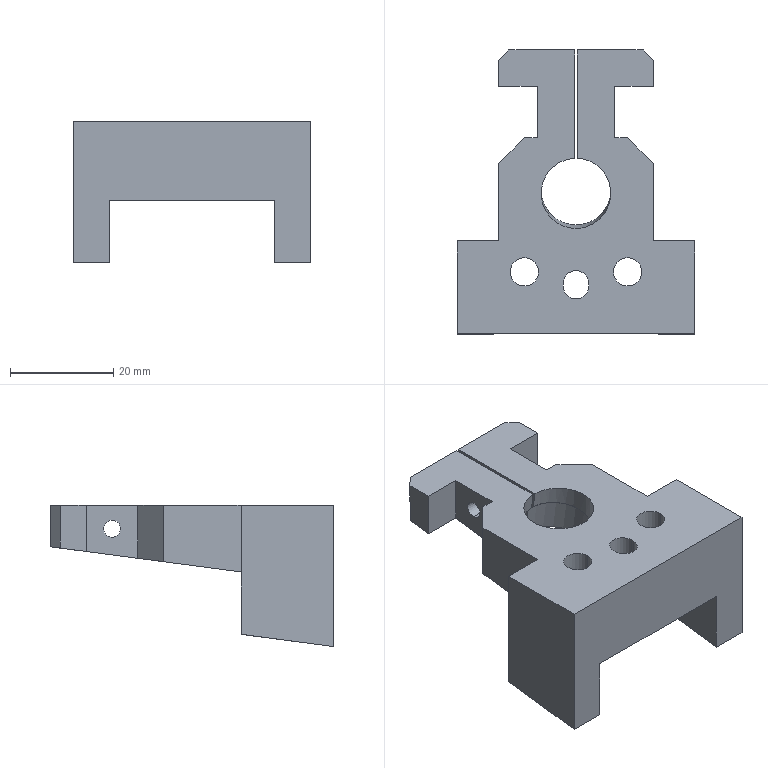Part | SolidWorks | features ICE 11, HoleWzd 5, Chamfer 3, Extrusion 1 | 1 solid | 79 faces | box 46 x 55 x 27.344 mm | volume 20060 mm3 | plane 34 | cylinder 30 | cone 15 | commonest cylinder face diameters 3.3 x10 2.5 x6 5.5 x4 9.5 x4 4.5 x2 5 x2